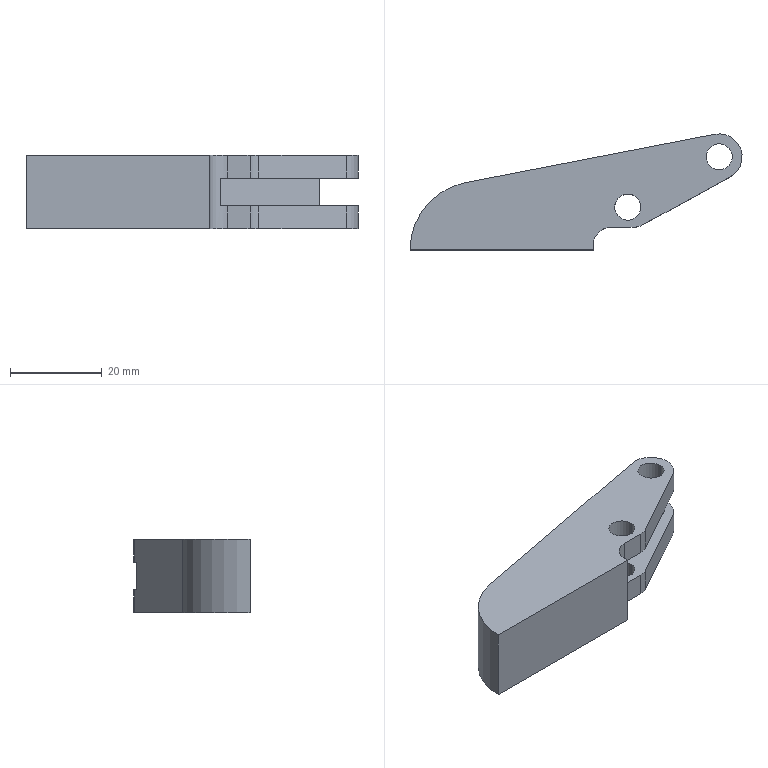Part | SolidWorks | features BaseBody 1, ICE 1, MoveFace 1 | 1 solid | 27 faces | box 72.59 x 25.381 x 16 mm | volume 14653 mm3 | cylinder 14 | plane 13 | commonest cylinder face diameters 5.7 x8 8 x3 10 x2 30 x1
STEP:
#1=CARTESIAN_POINT('',(70.44,20.381,5.));
#2=VERTEX_POINT('',#1);
#3=CARTESIAN_POINT('',(64.74,20.381,5.));
#4=VERTEX_POINT('',#3);
#5=CARTESIAN_POINT('',(67.59,20.381,5.));
#6=DIRECTION('',(0.,0.,-1.));
#7=DIRECTION('',(1.,0.,0.));
#8=AXIS2_PLACEMENT_3D('',#5,#6,#7);
#9=CIRCLE('',#8,2.85);
#10=EDGE_CURVE('',#2,#4,#9,.T.);
#11=ORIENTED_EDGE('',*,*,#10,.F.);
#12=CARTESIAN_POINT('',(70.44,20.381,0.));
#13=VERTEX_POINT('',#12);
#14=CARTESIAN_POINT('',(70.44,20.381,5.));
#15=DIRECTION('',(0.,0.,-1.));
#16=VECTOR('',#15,1000.);
#17=LINE('',#14,#16);
#18=EDGE_CURVE('',#2,#13,#17,.T.);
#19=ORIENTED_EDGE('',*,*,#18,.T.);
#20=CARTESIAN_POINT('',(64.74,20.381,0.));
#21=VERTEX_POINT('',#20);
#22=CARTESIAN_POINT('',(67.59,20.381,0.));
#23=DIRECTION('',(0.,0.,-1.));
#24=DIRECTION('',(1.,0.,0.));
#25=AXIS2_PLACEMENT_3D('',#22,#23,#24);
#26=CIRCLE('',#25,2.85);
#27=EDGE_CURVE('',#13,#21,#26,.T.);
#28=ORIENTED_EDGE('',*,*,#27,.T.);
#29=CARTESIAN_POINT('',(64.74,20.381,5.));
#30=DIRECTION('',(0.,0.,-1.));
#31=VECTOR('',#30,1000.);
#32=LINE('',#29,#31);
#33=EDGE_CURVE('',#4,#21,#32,.T.);
#34=ORIENTED_EDGE('',*,*,#33,.F.);
#35=EDGE_LOOP('',(#11,#19,#28,#34));
#36=FACE_OUTER_BOUND('',#35,.T.);
#37=CARTESIAN_POINT('',(67.59,20.381,5.));
#38=DIRECTION('',(0.,0.,-1.));
#39=DIRECTION('',(-1.,0.,0.));
#40=AXIS2_PLACEMENT_3D('',#37,#38,#39);
#41=CYLINDRICAL_SURFACE('',#40,2.85);
#42=ADVANCED_FACE('',(#36),#41,.F.);
#43=CARTESIAN_POINT('',(50.44,9.381,5.));
#44=VERTEX_POINT('',#43);
#45=CARTESIAN_POINT('',(44.74,9.381,5.));
#46=VERTEX_POINT('',#45);
#47=CARTESIAN_POINT('',(47.59,9.381,5.));
#48=DIRECTION('',(0.,0.,-1.));
#49=DIRECTION('',(1.,0.,0.));
#50=AXIS2_PLACEMENT_3D('',#47,#48,#49);
#51=CIRCLE('',#50,2.85);
#52=EDGE_CURVE('',#44,#46,#51,.T.);
#53=ORIENTED_EDGE('',*,*,#52,.F.);
#54=CARTESIAN_POINT('',(50.44,9.381,0.));
#55=VERTEX_POINT('',#54);
#56=CARTESIAN_POINT('',(50.44,9.381,5.));
#57=DIRECTION('',(0.,0.,-1.));
#58=VECTOR('',#57,1000.);
#59=LINE('',#56,#58);
#60=EDGE_CURVE('',#44,#55,#59,.T.);
#61=ORIENTED_EDGE('',*,*,#60,.T.);
#62=CARTESIAN_POINT('',(44.74,9.381,0.));
#63=VERTEX_POINT('',#62);
#64=CARTESIAN_POINT('',(47.59,9.381,0.));
#65=DIRECTION('',(0.,0.,-1.));
#66=DIRECTION('',(1.,0.,0.));
#67=AXIS2_PLACEMENT_3D('',#64,#65,#66);
#68=CIRCLE('',#67,2.85);
#69=EDGE_CURVE('',#55,#63,#68,.T.);
#70=ORIENTED_EDGE('',*,*,#69,.T.);
#71=CARTESIAN_POINT('',(44.74,9.381,5.));
#72=DIRECTION('',(0.,0.,-1.));
#73=VECTOR('',#72,1000.);
#74=LINE('',#71,#73);
#75=EDGE_CURVE('',#46,#63,#74,.T.);
#76=ORIENTED_EDGE('',*,*,#75,.F.);
#77=EDGE_LOOP('',(#53,#61,#70,#76));
#78=FACE_OUTER_BOUND('',#77,.T.);
#79=CARTESIAN_POINT('',(47.59,9.381,5.));
#80=DIRECTION('',(0.,0.,-1.));
#81=DIRECTION('',(-1.,0.,0.));
#82=AXIS2_PLACEMENT_3D('',#79,#80,#81);
#83=CYLINDRICAL_SURFACE('',#82,2.85);
#84=ADVANCED_FACE('',(#78),#83,.F.);
#85=CARTESIAN_POINT('',(64.74,20.381,16.));
#86=VERTEX_POINT('',#85);
#87=CARTESIAN_POINT('',(70.44,20.381,16.));
#88=VERTEX_POINT('',#87);
#89=CARTESIAN_POINT('',(67.59,20.381,16.));
#90=DIRECTION('',(0.,0.,1.));
#91=DIRECTION('',(1.,0.,0.));
#92=AXIS2_PLACEMENT_3D('',#89,#90,#91);
#93=CIRCLE('',#92,2.85);
#94=EDGE_CURVE('',#86,#88,#93,.T.);
#95=ORIENTED_EDGE('',*,*,#94,.T.);
#96=CARTESIAN_POINT('',(70.44,20.381,11.));
#97=VERTEX_POINT('',#96);
#98=CARTESIAN_POINT('',(70.44,20.381,16.));
#99=DIRECTION('',(0.,0.,-1.));
#100=VECTOR('',#99,1000.);
#101=LINE('',#98,#100);
#102=EDGE_CURVE('',#88,#97,#101,.T.);
#103=ORIENTED_EDGE('',*,*,#102,.T.);
#104=CARTESIAN_POINT('',(64.74,20.381,11.));
#105=VERTEX_POINT('',#104);
#106=CARTESIAN_POINT('',(67.59,20.381,11.));
#107=DIRECTION('',(0.,0.,-1.));
#108=DIRECTION('',(-1.,0.,0.));
#109=AXIS2_PLACEMENT_3D('',#106,#107,#108);
#110=CIRCLE('',#109,2.85);
#111=EDGE_CURVE('',#97,#105,#110,.T.);
#112=ORIENTED_EDGE('',*,*,#111,.T.);
#113=CARTESIAN_POINT('',(64.74,20.381,16.));
#114=DIRECTION('',(0.,0.,-1.));
#115=VECTOR('',#114,1000.);
#116=LINE('',#113,#115);
#117=EDGE_CURVE('',#86,#105,#116,.T.);
#118=ORIENTED_EDGE('',*,*,#117,.F.);
#119=EDGE_LOOP('',(#95,#103,#112,#118));
#120=FACE_OUTER_BOUND('',#119,.T.);
#121=CARTESIAN_POINT('',(67.59,20.381,16.));
#122=DIRECTION('',(0.,0.,-1.));
#123=DIRECTION('',(-1.,0.,0.));
#124=AXIS2_PLACEMENT_3D('',#121,#122,#123);
#125=CYLINDRICAL_SURFACE('',#124,2.85);
#126=ADVANCED_FACE('',(#120),#125,.F.);
#127=CARTESIAN_POINT('',(44.74,9.381,16.));
#128=VERTEX_POINT('',#127);
#129=CARTESIAN_POINT('',(50.44,9.381,16.));
#130=VERTEX_POINT('',#129);
#131=CARTESIAN_POINT('',(47.59,9.381,16.));
#132=DIRECTION('',(0.,0.,1.));
#133=DIRECTION('',(1.,0.,0.));
#134=AXIS2_PLACEMENT_3D('',#131,#132,#133);
#135=CIRCLE('',#134,2.85);
#136=EDGE_CURVE('',#128,#130,#135,.T.);
#137=ORIENTED_EDGE('',*,*,#136,.T.);
#138=CARTESIAN_POINT('',(50.44,9.381,11.));
#139=VERTEX_POINT('',#138);
#140=CARTESIAN_POINT('',(50.44,9.381,16.));
#141=DIRECTION('',(0.,0.,-1.));
#142=VECTOR('',#141,1000.);
#143=LINE('',#140,#142);
#144=EDGE_CURVE('',#130,#139,#143,.T.);
#145=ORIENTED_EDGE('',*,*,#144,.T.);
#146=CARTESIAN_POINT('',(44.74,9.381,11.));
#147=VERTEX_POINT('',#146);
#148=CARTESIAN_POINT('',(47.59,9.381,11.));
#149=DIRECTION('',(0.,0.,-1.));
#150=DIRECTION('',(-1.,0.,0.));
#151=AXIS2_PLACEMENT_3D('',#148,#149,#150);
#152=CIRCLE('',#151,2.85);
#153=EDGE_CURVE('',#139,#147,#152,.T.);
#154=ORIENTED_EDGE('',*,*,#153,.T.);
#155=CARTESIAN_POINT('',(44.74,9.381,16.));
#156=DIRECTION('',(0.,0.,-1.));
#157=VECTOR('',#156,1000.);
#158=LINE('',#155,#157);
#159=EDGE_CURVE('',#128,#147,#158,.T.);
#160=ORIENTED_EDGE('',*,*,#159,.F.);
#161=EDGE_LOOP('',(#137,#145,#154,#160));
#162=FACE_OUTER_BOUND('',#161,.T.);
#163=CARTESIAN_POINT('',(47.59,9.381,16.));
#164=DIRECTION('',(0.,0.,-1.));
#165=DIRECTION('',(-1.,0.,0.));
#166=AXIS2_PLACEMENT_3D('',#163,#164,#165);
#167=CYLINDRICAL_SURFACE('',#166,2.85);
#168=ADVANCED_FACE('',(#162),#167,.F.);
#169=CARTESIAN_POINT('',(42.59,12.922,5.));
#170=VERTEX_POINT('',#169);
#171=CARTESIAN_POINT('',(64.228,24.822,5.));
#172=VERTEX_POINT('',#171);
#173=CARTESIAN_POINT('',(45.834,14.706,5.));
#174=DIRECTION('',(0.8762,0.4819,0.));
#175=VECTOR('',#174,1000.);
#176=LINE('',#173,#175);
#177=EDGE_CURVE('',#170,#172,#176,.T.);
#178=ORIENTED_EDGE('',*,*,#177,.T.);
#179=CARTESIAN_POINT('',(64.228,24.822,11.));
#180=VERTEX_POINT('',#179);
#181=CARTESIAN_POINT('',(64.228,24.822,16.));
#182=DIRECTION('',(0.,0.,1.));
#183=VECTOR('',#182,1000.);
#184=LINE('',#181,#183);
#185=EDGE_CURVE('',#172,#180,#184,.T.);
#186=ORIENTED_EDGE('',*,*,#185,.T.);
#187=CARTESIAN_POINT('',(42.59,12.922,11.));
#188=VERTEX_POINT('',#187);
#189=CARTESIAN_POINT('',(86.688,37.175,11.));
#190=DIRECTION('',(0.8762,0.4819,0.));
#191=VECTOR('',#190,1000.);
#192=LINE('',#189,#191);
#193=EDGE_CURVE('',#188,#180,#192,.T.);
#194=ORIENTED_EDGE('',*,*,#193,.F.);
#195=CARTESIAN_POINT('',(42.59,12.922,11.));
#196=DIRECTION('',(0.,0.,1.));
#197=VECTOR('',#196,1000.);
#198=LINE('',#195,#197);
#199=EDGE_CURVE('',#170,#188,#198,.T.);
#200=ORIENTED_EDGE('',*,*,#199,.F.);
#201=EDGE_LOOP('',(#178,#186,#194,#200));
#202=FACE_OUTER_BOUND('',#201,.T.);
#203=CARTESIAN_POINT('',(45.834,14.706,16.));
#204=DIRECTION('',(-0.4819,0.8762,0.));
#205=DIRECTION('',(-0.8762,-0.4819,0.));
#206=AXIS2_PLACEMENT_3D('',#203,#204,#205);
#207=PLANE('',#206);
#208=ADVANCED_FACE('',(#202),#207,.F.);
#209=CARTESIAN_POINT('',(47.59,9.381,11.));
#210=DIRECTION('',(0.,0.,-1.));
#211=DIRECTION('',(-1.,0.,0.));
#212=AXIS2_PLACEMENT_3D('',#209,#210,#211);
#213=CIRCLE('',#212,2.85);
#214=EDGE_CURVE('',#147,#139,#213,.T.);
#215=ORIENTED_EDGE('',*,*,#214,.F.);
#216=ORIENTED_EDGE('',*,*,#153,.F.);
#217=EDGE_LOOP('',(#215,#216));
#218=FACE_BOUND('',#217,.T.);
#219=CARTESIAN_POINT('',(67.59,20.381,11.));
#220=DIRECTION('',(0.,0.,-1.));
#221=DIRECTION('',(-1.,0.,0.));
#222=AXIS2_PLACEMENT_3D('',#219,#220,#221);
#223=CIRCLE('',#222,2.85);
#224=EDGE_CURVE('',#105,#97,#223,.T.);
#225=ORIENTED_EDGE('',*,*,#224,.F.);
#226=ORIENTED_EDGE('',*,*,#111,.F.);
#227=EDGE_LOOP('',(#225,#226));
#228=FACE_BOUND('',#227,.T.);
#229=CARTESIAN_POINT('',(66.639,25.29,11.));
#230=VERTEX_POINT('',#229);
#231=CARTESIAN_POINT('',(12.145,14.726,11.));
#232=DIRECTION('',(-0.9817,-0.1903,0.));
#233=VECTOR('',#232,1000.);
#234=LINE('',#231,#233);
#235=EDGE_CURVE('',#230,#180,#234,.T.);
#236=ORIENTED_EDGE('',*,*,#235,.F.);
#237=CARTESIAN_POINT('',(70.,16.,11.));
#238=VERTEX_POINT('',#237);
#239=CARTESIAN_POINT('',(67.59,20.381,11.));
#240=DIRECTION('',(0.,0.,1.));
#241=DIRECTION('',(-1.,0.,0.));
#242=AXIS2_PLACEMENT_3D('',#239,#240,#241);
#243=CIRCLE('',#242,5.);
#244=EDGE_CURVE('',#238,#230,#243,.T.);
#245=ORIENTED_EDGE('',*,*,#244,.F.);
#246=CARTESIAN_POINT('',(50.9,5.495,11.));
#247=VERTEX_POINT('',#246);
#248=CARTESIAN_POINT('',(50.9,5.495,11.));
#249=DIRECTION('',(-0.8762,-0.4819,0.));
#250=VECTOR('',#249,1000.);
#251=LINE('',#248,#250);
#252=EDGE_CURVE('',#238,#247,#251,.T.);
#253=ORIENTED_EDGE('',*,*,#252,.T.);
#254=CARTESIAN_POINT('',(48.973,5.,11.));
#255=VERTEX_POINT('',#254);
#256=CARTESIAN_POINT('',(48.973,9.,11.));
#257=DIRECTION('',(0.,0.,1.));
#258=DIRECTION('',(-1.,0.,0.));
#259=AXIS2_PLACEMENT_3D('',#256,#257,#258);
#260=CIRCLE('',#259,4.);
#261=EDGE_CURVE('',#255,#247,#260,.T.);
#262=ORIENTED_EDGE('',*,*,#261,.F.);
#263=CARTESIAN_POINT('',(44.,5.,11.));
#264=VERTEX_POINT('',#263);
#265=CARTESIAN_POINT('',(44.,5.,11.));
#266=DIRECTION('',(-1.,0.,0.));
#267=VECTOR('',#266,1000.);
#268=LINE('',#265,#267);
#269=EDGE_CURVE('',#255,#264,#268,.T.);
#270=ORIENTED_EDGE('',*,*,#269,.T.);
#271=CARTESIAN_POINT('',(42.59,4.743,11.));
#272=VERTEX_POINT('',#271);
#273=CARTESIAN_POINT('',(44.,1.,11.));
#274=DIRECTION('',(0.,0.,1.));
#275=DIRECTION('',(-1.,0.,0.));
#276=AXIS2_PLACEMENT_3D('',#273,#274,#275);
#277=CIRCLE('',#276,4.);
#278=EDGE_CURVE('',#264,#272,#277,.T.);
#279=ORIENTED_EDGE('',*,*,#278,.T.);
#280=CARTESIAN_POINT('',(42.59,62.807,11.));
#281=DIRECTION('',(0.,-1.,0.));
#282=VECTOR('',#281,1000.);
#283=LINE('',#280,#282);
#284=EDGE_CURVE('',#188,#272,#283,.T.);
#285=ORIENTED_EDGE('',*,*,#284,.F.);
#286=ORIENTED_EDGE('',*,*,#193,.T.);
#287=EDGE_LOOP('',(#236,#245,#253,#262,#270,#279,#285,#286));
#288=FACE_OUTER_BOUND('',#287,.T.);
#289=CARTESIAN_POINT('',(72.59,62.807,11.));
#290=DIRECTION('',(0.,0.,-1.));
#291=DIRECTION('',(-1.,0.,0.));
#292=AXIS2_PLACEMENT_3D('',#289,#290,#291);
#293=PLANE('',#292);
#294=ADVANCED_FACE('',(#218,#228,#288),#293,.T.);
#295=CARTESIAN_POINT('',(67.59,20.381,5.));
#296=DIRECTION('',(0.,0.,-1.));
#297=DIRECTION('',(1.,0.,0.));
#298=AXIS2_PLACEMENT_3D('',#295,#296,#297);
#299=CIRCLE('',#298,2.85);
#300=EDGE_CURVE('',#4,#2,#299,.T.);
#301=ORIENTED_EDGE('',*,*,#300,.T.);
#302=ORIENTED_EDGE('',*,*,#10,.T.);
#303=EDGE_LOOP('',(#301,#302));
#304=FACE_BOUND('',#303,.T.);
#305=CARTESIAN_POINT('',(47.59,9.381,5.));
#306=DIRECTION('',(0.,0.,-1.));
#307=DIRECTION('',(1.,0.,0.));
#308=AXIS2_PLACEMENT_3D('',#305,#306,#307);
#309=CIRCLE('',#308,2.85);
#310=EDGE_CURVE('',#46,#44,#309,.T.);
#311=ORIENTED_EDGE('',*,*,#310,.T.);
#312=ORIENTED_EDGE('',*,*,#52,.T.);
#313=EDGE_LOOP('',(#311,#312));
#314=FACE_BOUND('',#313,.T.);
#315=CARTESIAN_POINT('',(66.639,25.29,5.));
#316=VERTEX_POINT('',#315);
#317=CARTESIAN_POINT('',(70.,16.,5.));
#318=VERTEX_POINT('',#317);
#319=CARTESIAN_POINT('',(67.59,20.381,5.));
#320=DIRECTION('',(0.,0.,-1.));
#321=DIRECTION('',(-1.,0.,0.));
#322=AXIS2_PLACEMENT_3D('',#319,#320,#321);
#323=CIRCLE('',#322,5.);
#324=EDGE_CURVE('',#316,#318,#323,.T.);
#325=ORIENTED_EDGE('',*,*,#324,.F.);
#326=CARTESIAN_POINT('',(40.282,20.18,5.));
#327=DIRECTION('',(-0.9817,-0.1903,0.));
#328=VECTOR('',#327,1000.);
#329=LINE('',#326,#328);
#330=EDGE_CURVE('',#316,#172,#329,.T.);
#331=ORIENTED_EDGE('',*,*,#330,.T.);
#332=ORIENTED_EDGE('',*,*,#177,.F.);
#333=CARTESIAN_POINT('',(42.59,4.743,5.));
#334=VERTEX_POINT('',#333);
#335=CARTESIAN_POINT('',(42.59,4.743,5.));
#336=DIRECTION('',(0.,1.,0.));
#337=VECTOR('',#336,1000.);
#338=LINE('',#335,#337);
#339=EDGE_CURVE('',#334,#170,#338,.T.);
#340=ORIENTED_EDGE('',*,*,#339,.F.);
#341=CARTESIAN_POINT('',(44.,5.,5.));
#342=VERTEX_POINT('',#341);
#343=CARTESIAN_POINT('',(44.,1.,5.));
#344=DIRECTION('',(0.,0.,1.));
#345=DIRECTION('',(1.,0.,0.));
#346=AXIS2_PLACEMENT_3D('',#343,#344,#345);
#347=CIRCLE('',#346,4.);
#348=EDGE_CURVE('',#342,#334,#347,.T.);
#349=ORIENTED_EDGE('',*,*,#348,.F.);
#350=CARTESIAN_POINT('',(48.973,5.,5.));
#351=VERTEX_POINT('',#350);
#352=CARTESIAN_POINT('',(48.973,5.,5.));
#353=DIRECTION('',(-1.,0.,0.));
#354=VECTOR('',#353,1000.);
#355=LINE('',#352,#354);
#356=EDGE_CURVE('',#351,#342,#355,.T.);
#357=ORIENTED_EDGE('',*,*,#356,.F.);
#358=CARTESIAN_POINT('',(50.9,5.495,5.));
#359=VERTEX_POINT('',#358);
#360=CARTESIAN_POINT('',(48.973,9.,5.));
#361=DIRECTION('',(0.,0.,-1.));
#362=DIRECTION('',(-1.,0.,0.));
#363=AXIS2_PLACEMENT_3D('',#360,#361,#362);
#364=CIRCLE('',#363,4.);
#365=EDGE_CURVE('',#359,#351,#364,.T.);
#366=ORIENTED_EDGE('',*,*,#365,.F.);
#367=CARTESIAN_POINT('',(70.,16.,5.));
#368=DIRECTION('',(-0.8762,-0.4819,0.));
#369=VECTOR('',#368,1000.);
#370=LINE('',#367,#369);
#371=EDGE_CURVE('',#318,#359,#370,.T.);
#372=ORIENTED_EDGE('',*,*,#371,.F.);
#373=EDGE_LOOP('',(#325,#331,#332,#340,#349,#357,#366,#372));
#374=FACE_OUTER_BOUND('',#373,.T.);
#375=CARTESIAN_POINT('',(44.,1.,5.));
#376=DIRECTION('',(0.,0.,1.));
#377=DIRECTION('',(1.,0.,0.));
#378=AXIS2_PLACEMENT_3D('',#375,#376,#377);
#379=PLANE('',#378);
#380=ADVANCED_FACE('',(#304,#314,#374),#379,.T.);
#381=ORIENTED_EDGE('',*,*,#244,.T.);
#382=CARTESIAN_POINT('',(66.639,25.29,16.));
#383=VERTEX_POINT('',#382);
#384=CARTESIAN_POINT('',(66.639,25.29,16.));
#385=DIRECTION('',(0.,0.,-1.));
#386=VECTOR('',#385,1000.);
#387=LINE('',#384,#386);
#388=EDGE_CURVE('',#383,#230,#387,.T.);
#389=ORIENTED_EDGE('',*,*,#388,.F.);
#390=CARTESIAN_POINT('',(70.,16.,16.));
#391=VERTEX_POINT('',#390);
#392=CARTESIAN_POINT('',(67.59,20.381,16.));
#393=DIRECTION('',(0.,0.,-1.));
#394=DIRECTION('',(-1.,0.,0.));
#395=AXIS2_PLACEMENT_3D('',#392,#393,#394);
#396=CIRCLE('',#395,5.);
#397=EDGE_CURVE('',#383,#391,#396,.T.);
#398=ORIENTED_EDGE('',*,*,#397,.T.);
#399=CARTESIAN_POINT('',(70.,16.,16.));
#400=DIRECTION('',(0.,0.,-1.));
#401=VECTOR('',#400,1000.);
#402=LINE('',#399,#401);
#403=EDGE_CURVE('',#391,#238,#402,.T.);
#404=ORIENTED_EDGE('',*,*,#403,.T.);
#405=EDGE_LOOP('',(#381,#389,#398,#404));
#406=FACE_OUTER_BOUND('',#405,.T.);
#407=CARTESIAN_POINT('',(67.59,20.381,16.));
#408=DIRECTION('',(0.,0.,-1.));
#409=DIRECTION('',(-1.,0.,0.));
#410=AXIS2_PLACEMENT_3D('',#407,#408,#409);
#411=CYLINDRICAL_SURFACE('',#410,5.);
#412=ADVANCED_FACE('',(#406),#411,.T.);
#413=CARTESIAN_POINT('',(40.,1.,0.));
#414=VERTEX_POINT('',#413);
#415=CARTESIAN_POINT('',(44.,5.,0.));
#416=VERTEX_POINT('',#415);
#417=CARTESIAN_POINT('',(44.,1.,0.));
#418=DIRECTION('',(0.,0.,-1.));
#419=DIRECTION('',(-1.,0.,0.));
#420=AXIS2_PLACEMENT_3D('',#417,#418,#419);
#421=CIRCLE('',#420,4.);
#422=EDGE_CURVE('',#414,#416,#421,.T.);
#423=ORIENTED_EDGE('',*,*,#422,.T.);
#424=CARTESIAN_POINT('',(44.,5.,5.));
#425=DIRECTION('',(0.,0.,-1.));
#426=VECTOR('',#425,1000.);
#427=LINE('',#424,#426);
#428=EDGE_CURVE('',#342,#416,#427,.T.);
#429=ORIENTED_EDGE('',*,*,#428,.F.);
#430=ORIENTED_EDGE('',*,*,#348,.T.);
#431=CARTESIAN_POINT('',(42.59,4.743,16.));
#432=DIRECTION('',(0.,0.,-1.));
#433=VECTOR('',#432,1000.);
#434=LINE('',#431,#433);
#435=EDGE_CURVE('',#272,#334,#434,.T.);
#436=ORIENTED_EDGE('',*,*,#435,.F.);
#437=ORIENTED_EDGE('',*,*,#278,.F.);
#438=CARTESIAN_POINT('',(44.,5.,16.));
#439=VERTEX_POINT('',#438);
#440=CARTESIAN_POINT('',(44.,5.,16.));
#441=DIRECTION('',(0.,0.,-1.));
#442=VECTOR('',#441,1000.);
#443=LINE('',#440,#442);
#444=EDGE_CURVE('',#439,#264,#443,.T.);
#445=ORIENTED_EDGE('',*,*,#444,.F.);
#446=CARTESIAN_POINT('',(40.,1.,16.));
#447=VERTEX_POINT('',#446);
#448=CARTESIAN_POINT('',(44.,1.,16.));
#449=DIRECTION('',(0.,0.,-1.));
#450=DIRECTION('',(-1.,0.,0.));
#451=AXIS2_PLACEMENT_3D('',#448,#449,#450);
#452=CIRCLE('',#451,4.);
#453=EDGE_CURVE('',#447,#439,#452,.T.);
#454=ORIENTED_EDGE('',*,*,#453,.F.);
#455=CARTESIAN_POINT('',(40.,1.,16.));
#456=DIRECTION('',(0.,0.,-1.));
#457=VECTOR('',#456,1000.);
#458=LINE('',#455,#457);
#459=EDGE_CURVE('',#447,#414,#458,.T.);
#460=ORIENTED_EDGE('',*,*,#459,.T.);
#461=EDGE_LOOP('',(#423,#429,#430,#436,#437,#445,#454,#460));
#462=FACE_OUTER_BOUND('',#461,.T.);
#463=CARTESIAN_POINT('',(44.,1.,16.));
#464=DIRECTION('',(0.,0.,-1.));
#465=DIRECTION('',(-1.,0.,0.));
#466=AXIS2_PLACEMENT_3D('',#463,#464,#465);
#467=CYLINDRICAL_SURFACE('',#466,4.);
#468=ADVANCED_FACE('',(#462),#467,.F.);
#469=ORIENTED_EDGE('',*,*,#269,.F.);
#470=CARTESIAN_POINT('',(48.973,5.,16.));
#471=VERTEX_POINT('',#470);
#472=CARTESIAN_POINT('',(48.973,5.,16.));
#473=DIRECTION('',(0.,0.,-1.));
#474=VECTOR('',#473,1000.);
#475=LINE('',#472,#474);
#476=EDGE_CURVE('',#471,#255,#475,.T.);
#477=ORIENTED_EDGE('',*,*,#476,.F.);
#478=CARTESIAN_POINT('',(44.,5.,16.));
#479=DIRECTION('',(1.,0.,0.));
#480=VECTOR('',#479,1000.);
#481=LINE('',#478,#480);
#482=EDGE_CURVE('',#439,#471,#481,.T.);
#483=ORIENTED_EDGE('',*,*,#482,.F.);
#484=ORIENTED_EDGE('',*,*,#444,.T.);
#485=EDGE_LOOP('',(#469,#477,#483,#484));
#486=FACE_OUTER_BOUND('',#485,.T.);
#487=CARTESIAN_POINT('',(44.,5.,16.));
#488=DIRECTION('',(0.,1.,0.));
#489=DIRECTION('',(-1.,0.,0.));
#490=AXIS2_PLACEMENT_3D('',#487,#488,#489);
#491=PLANE('',#490);
#492=ADVANCED_FACE('',(#486),#491,.F.);
#493=ORIENTED_EDGE('',*,*,#476,.T.);
#494=ORIENTED_EDGE('',*,*,#261,.T.);
#495=CARTESIAN_POINT('',(50.9,5.495,16.));
#496=VERTEX_POINT('',#495);
#497=CARTESIAN_POINT('',(50.9,5.495,16.));
#498=DIRECTION('',(0.,0.,-1.));
#499=VECTOR('',#498,1000.);
#500=LINE('',#497,#499);
#501=EDGE_CURVE('',#496,#247,#500,.T.);
#502=ORIENTED_EDGE('',*,*,#501,.F.);
#503=CARTESIAN_POINT('',(48.973,9.,16.));
#504=DIRECTION('',(0.,0.,-1.));
#505=DIRECTION('',(-1.,0.,0.));
#506=AXIS2_PLACEMENT_3D('',#503,#504,#505);
#507=CIRCLE('',#506,4.);
#508=EDGE_CURVE('',#496,#471,#507,.T.);
#509=ORIENTED_EDGE('',*,*,#508,.T.);
#510=EDGE_LOOP('',(#493,#494,#502,#509));
#511=FACE_OUTER_BOUND('',#510,.T.);
#512=CARTESIAN_POINT('',(48.973,9.,16.));
#513=DIRECTION('',(0.,0.,-1.));
#514=DIRECTION('',(-1.,0.,0.));
#515=AXIS2_PLACEMENT_3D('',#512,#513,#514);
#516=CYLINDRICAL_SURFACE('',#515,4.);
#517=ADVANCED_FACE('',(#511),#516,.T.);
#518=ORIENTED_EDGE('',*,*,#252,.F.);
#519=ORIENTED_EDGE('',*,*,#403,.F.);
#520=CARTESIAN_POINT('',(50.9,5.495,16.));
#521=DIRECTION('',(0.8762,0.4819,0.));
#522=VECTOR('',#521,1000.);
#523=LINE('',#520,#522);
#524=EDGE_CURVE('',#496,#391,#523,.T.);
#525=ORIENTED_EDGE('',*,*,#524,.F.);
#526=ORIENTED_EDGE('',*,*,#501,.T.);
#527=EDGE_LOOP('',(#518,#519,#525,#526));
#528=FACE_OUTER_BOUND('',#527,.T.);
#529=CARTESIAN_POINT('',(50.9,5.495,16.));
#530=DIRECTION('',(-0.4819,0.8762,0.));
#531=DIRECTION('',(-0.8762,-0.4819,0.));
#532=AXIS2_PLACEMENT_3D('',#529,#530,#531);
#533=PLANE('',#532);
#534=ADVANCED_FACE('',(#528),#533,.F.);
#535=CARTESIAN_POINT('',(66.639,25.29,0.));
#536=VERTEX_POINT('',#535);
#537=CARTESIAN_POINT('',(66.639,25.29,16.));
#538=DIRECTION('',(0.,0.,-1.));
#539=VECTOR('',#538,1000.);
#540=LINE('',#537,#539);
#541=EDGE_CURVE('',#316,#536,#540,.T.);
#542=ORIENTED_EDGE('',*,*,#541,.F.);
#543=ORIENTED_EDGE('',*,*,#324,.T.);
#544=CARTESIAN_POINT('',(70.,16.,0.));
#545=VERTEX_POINT('',#544);
#546=CARTESIAN_POINT('',(70.,16.,5.));
#547=DIRECTION('',(0.,0.,-1.));
#548=VECTOR('',#547,1000.);
#549=LINE('',#546,#548);
#550=EDGE_CURVE('',#318,#545,#549,.T.);
#551=ORIENTED_EDGE('',*,*,#550,.T.);
#552=CARTESIAN_POINT('',(67.59,20.381,0.));
#553=DIRECTION('',(0.,0.,-1.));
#554=DIRECTION('',(-1.,0.,0.));
#555=AXIS2_PLACEMENT_3D('',#552,#553,#554);
#556=CIRCLE('',#555,5.);
#557=EDGE_CURVE('',#536,#545,#556,.T.);
#558=ORIENTED_EDGE('',*,*,#557,.F.);
#559=EDGE_LOOP('',(#542,#543,#551,#558));
#560=FACE_OUTER_BOUND('',#559,.T.);
#561=CARTESIAN_POINT('',(67.59,20.381,16.));
#562=DIRECTION('',(0.,0.,-1.));
#563=DIRECTION('',(-1.,0.,0.));
#564=AXIS2_PLACEMENT_3D('',#561,#562,#563);
#565=CYLINDRICAL_SURFACE('',#564,5.);
#566=ADVANCED_FACE('',(#560),#565,.T.);
#567=ORIENTED_EDGE('',*,*,#144,.F.);
#568=CARTESIAN_POINT('',(47.59,9.381,16.));
#569=DIRECTION('',(0.,0.,1.));
#570=DIRECTION('',(1.,0.,0.));
#571=AXIS2_PLACEMENT_3D('',#568,#569,#570);
#572=CIRCLE('',#571,2.85);
#573=EDGE_CURVE('',#130,#128,#572,.T.);
#574=ORIENTED_EDGE('',*,*,#573,.T.);
#575=ORIENTED_EDGE('',*,*,#159,.T.);
#576=ORIENTED_EDGE('',*,*,#214,.T.);
#577=EDGE_LOOP('',(#567,#574,#575,#576));
#578=FACE_OUTER_BOUND('',#577,.T.);
#579=CARTESIAN_POINT('',(47.59,9.381,16.));
#580=DIRECTION('',(0.,0.,-1.));
#581=DIRECTION('',(-1.,0.,0.));
#582=AXIS2_PLACEMENT_3D('',#579,#580,#581);
#583=CYLINDRICAL_SURFACE('',#582,2.85);
#584=ADVANCED_FACE('',(#578),#583,.F.);
#585=ORIENTED_EDGE('',*,*,#102,.F.);
#586=CARTESIAN_POINT('',(67.59,20.381,16.));
#587=DIRECTION('',(0.,0.,1.));
#588=DIRECTION('',(1.,0.,0.));
#589=AXIS2_PLACEMENT_3D('',#586,#587,#588);
#590=CIRCLE('',#589,2.85);
#591=EDGE_CURVE('',#88,#86,#590,.T.);
#592=ORIENTED_EDGE('',*,*,#591,.T.);
#593=ORIENTED_EDGE('',*,*,#117,.T.);
#594=ORIENTED_EDGE('',*,*,#224,.T.);
#595=EDGE_LOOP('',(#585,#592,#593,#594));
#596=FACE_OUTER_BOUND('',#595,.T.);
#597=CARTESIAN_POINT('',(67.59,20.381,16.));
#598=DIRECTION('',(0.,0.,-1.));
#599=DIRECTION('',(-1.,0.,0.));
#600=AXIS2_PLACEMENT_3D('',#597,#598,#599);
#601=CYLINDRICAL_SURFACE('',#600,2.85);
#602=ADVANCED_FACE('',(#596),#601,.F.);
#603=ORIENTED_EDGE('',*,*,#136,.F.);
#604=ORIENTED_EDGE('',*,*,#573,.F.);
#605=EDGE_LOOP('',(#603,#604));
#606=FACE_BOUND('',#605,.T.);
#607=CARTESIAN_POINT('',(12.145,14.726,16.));
#608=VERTEX_POINT('',#607);
#609=CARTESIAN_POINT('',(0.,0.,16.));
#610=VERTEX_POINT('',#609);
#611=CARTESIAN_POINT('',(15.,0.,16.));
#612=DIRECTION('',(0.,0.,1.));
#613=DIRECTION('',(1.,0.,0.));
#614=AXIS2_PLACEMENT_3D('',#611,#612,#613);
#615=CIRCLE('',#614,15.);
#616=EDGE_CURVE('',#608,#610,#615,.T.);
#617=ORIENTED_EDGE('',*,*,#616,.T.);
#618=CARTESIAN_POINT('',(40.,0.,16.));
#619=VERTEX_POINT('',#618);
#620=CARTESIAN_POINT('',(0.,0.,16.));
#621=DIRECTION('',(1.,0.,0.));
#622=VECTOR('',#621,1000.);
#623=LINE('',#620,#622);
#624=EDGE_CURVE('',#610,#619,#623,.T.);
#625=ORIENTED_EDGE('',*,*,#624,.T.);
#626=CARTESIAN_POINT('',(40.,0.,16.));
#627=DIRECTION('',(0.,1.,0.));
#628=VECTOR('',#627,1000.);
#629=LINE('',#626,#628);
#630=EDGE_CURVE('',#619,#447,#629,.T.);
#631=ORIENTED_EDGE('',*,*,#630,.T.);
#632=ORIENTED_EDGE('',*,*,#453,.T.);
#633=ORIENTED_EDGE('',*,*,#482,.T.);
#634=ORIENTED_EDGE('',*,*,#508,.F.);
#635=ORIENTED_EDGE('',*,*,#524,.T.);
#636=ORIENTED_EDGE('',*,*,#397,.F.);
#637=CARTESIAN_POINT('',(12.145,14.726,16.));
#638=DIRECTION('',(0.9817,0.1903,0.));
#639=VECTOR('',#638,1000.);
#640=LINE('',#637,#639);
#641=EDGE_CURVE('',#608,#383,#640,.T.);
#642=ORIENTED_EDGE('',*,*,#641,.F.);
#643=EDGE_LOOP('',(#617,#625,#631,#632,#633,#634,#635,#636,#642));
#644=FACE_OUTER_BOUND('',#643,.T.);
#645=ORIENTED_EDGE('',*,*,#94,.F.);
#646=ORIENTED_EDGE('',*,*,#591,.F.);
#647=EDGE_LOOP('',(#645,#646));
#648=FACE_BOUND('',#647,.T.);
#649=CARTESIAN_POINT('',(15.,0.,16.));
#650=DIRECTION('',(0.,0.,1.));
#651=DIRECTION('',(1.,0.,0.));
#652=AXIS2_PLACEMENT_3D('',#649,#650,#651);
#653=PLANE('',#652);
#654=ADVANCED_FACE('',(#606,#644,#648),#653,.T.);
#655=CARTESIAN_POINT('',(48.973,5.,0.));
#656=VERTEX_POINT('',#655);
#657=CARTESIAN_POINT('',(48.973,5.,0.));
#658=DIRECTION('',(-1.,0.,0.));
#659=VECTOR('',#658,1000.);
#660=LINE('',#657,#659);
#661=EDGE_CURVE('',#656,#416,#660,.T.);
#662=ORIENTED_EDGE('',*,*,#661,.T.);
#663=ORIENTED_EDGE('',*,*,#422,.F.);
#664=CARTESIAN_POINT('',(40.,0.,0.));
#665=VERTEX_POINT('',#664);
#666=CARTESIAN_POINT('',(40.,0.,0.));
#667=DIRECTION('',(0.,1.,0.));
#668=VECTOR('',#667,1000.);
#669=LINE('',#666,#668);
#670=EDGE_CURVE('',#665,#414,#669,.T.);
#671=ORIENTED_EDGE('',*,*,#670,.F.);
#672=CARTESIAN_POINT('',(0.,0.,0.));
#673=VERTEX_POINT('',#672);
#674=CARTESIAN_POINT('',(0.,0.,0.));
#675=DIRECTION('',(1.,0.,0.));
#676=VECTOR('',#675,1000.);
#677=LINE('',#674,#676);
#678=EDGE_CURVE('',#673,#665,#677,.T.);
#679=ORIENTED_EDGE('',*,*,#678,.F.);
#680=CARTESIAN_POINT('',(12.145,14.726,0.));
#681=VERTEX_POINT('',#680);
#682=CARTESIAN_POINT('',(15.,0.,0.));
#683=DIRECTION('',(0.,0.,1.));
#684=DIRECTION('',(1.,0.,0.));
#685=AXIS2_PLACEMENT_3D('',#682,#683,#684);
#686=CIRCLE('',#685,15.);
#687=EDGE_CURVE('',#681,#673,#686,.T.);
#688=ORIENTED_EDGE('',*,*,#687,.F.);
#689=CARTESIAN_POINT('',(12.145,14.726,0.));
#690=DIRECTION('',(0.9817,0.1903,0.));
#691=VECTOR('',#690,1000.);
#692=LINE('',#689,#691);
#693=EDGE_CURVE('',#681,#536,#692,.T.);
#694=ORIENTED_EDGE('',*,*,#693,.T.);
#695=ORIENTED_EDGE('',*,*,#557,.T.);
#696=CARTESIAN_POINT('',(50.9,5.495,0.));
#697=VERTEX_POINT('',#696);
#698=CARTESIAN_POINT('',(70.,16.,0.));
#699=DIRECTION('',(-0.8762,-0.4819,0.));
#700=VECTOR('',#699,1000.);
#701=LINE('',#698,#700);
#702=EDGE_CURVE('',#545,#697,#701,.T.);
#703=ORIENTED_EDGE('',*,*,#702,.T.);
#704=CARTESIAN_POINT('',(48.973,9.,0.));
#705=DIRECTION('',(0.,0.,-1.));
#706=DIRECTION('',(-1.,0.,0.));
#707=AXIS2_PLACEMENT_3D('',#704,#705,#706);
#708=CIRCLE('',#707,4.);
#709=EDGE_CURVE('',#697,#656,#708,.T.);
#710=ORIENTED_EDGE('',*,*,#709,.T.);
#711=EDGE_LOOP('',(#662,#663,#671,#679,#688,#694,#695,#703,#710));
#712=FACE_OUTER_BOUND('',#711,.T.);
#713=CARTESIAN_POINT('',(67.59,20.381,0.));
#714=DIRECTION('',(0.,0.,-1.));
#715=DIRECTION('',(1.,0.,0.));
#716=AXIS2_PLACEMENT_3D('',#713,#714,#715);
#717=CIRCLE('',#716,2.85);
#718=EDGE_CURVE('',#21,#13,#717,.T.);
#719=ORIENTED_EDGE('',*,*,#718,.F.);
#720=ORIENTED_EDGE('',*,*,#27,.F.);
#721=EDGE_LOOP('',(#719,#720));
#722=FACE_BOUND('',#721,.T.);
#723=CARTESIAN_POINT('',(47.59,9.381,0.));
#724=DIRECTION('',(0.,0.,-1.));
#725=DIRECTION('',(1.,0.,0.));
#726=AXIS2_PLACEMENT_3D('',#723,#724,#725);
#727=CIRCLE('',#726,2.85);
#728=EDGE_CURVE('',#63,#55,#727,.T.);
#729=ORIENTED_EDGE('',*,*,#728,.F.);
#730=ORIENTED_EDGE('',*,*,#69,.F.);
#731=EDGE_LOOP('',(#729,#730));
#732=FACE_BOUND('',#731,.T.);
#733=CARTESIAN_POINT('',(15.,0.,0.));
#734=DIRECTION('',(0.,0.,1.));
#735=DIRECTION('',(1.,0.,0.));
#736=AXIS2_PLACEMENT_3D('',#733,#734,#735);
#737=PLANE('',#736);
#738=ADVANCED_FACE('',(#712,#722,#732),#737,.F.);
#739=ORIENTED_EDGE('',*,*,#687,.T.);
#740=CARTESIAN_POINT('',(0.,0.,16.));
#741=DIRECTION('',(0.,0.,-1.));
#742=VECTOR('',#741,1000.);
#743=LINE('',#740,#742);
#744=EDGE_CURVE('',#610,#673,#743,.T.);
#745=ORIENTED_EDGE('',*,*,#744,.F.);
#746=ORIENTED_EDGE('',*,*,#616,.F.);
#747=CARTESIAN_POINT('',(12.145,14.726,16.));
#748=DIRECTION('',(0.,0.,-1.));
#749=VECTOR('',#748,1000.);
#750=LINE('',#747,#749);
#751=EDGE_CURVE('',#608,#681,#750,.T.);
#752=ORIENTED_EDGE('',*,*,#751,.T.);
#753=EDGE_LOOP('',(#739,#745,#746,#752));
#754=FACE_OUTER_BOUND('',#753,.T.);
#755=CARTESIAN_POINT('',(15.,0.,16.));
#756=DIRECTION('',(0.,0.,-1.));
#757=DIRECTION('',(-1.,0.,0.));
#758=AXIS2_PLACEMENT_3D('',#755,#756,#757);
#759=CYLINDRICAL_SURFACE('',#758,15.);
#760=ADVANCED_FACE('',(#754),#759,.T.);
#761=ORIENTED_EDGE('',*,*,#678,.T.);
#762=CARTESIAN_POINT('',(40.,0.,16.));
#763=DIRECTION('',(0.,0.,-1.));
#764=VECTOR('',#763,1000.);
#765=LINE('',#762,#764);
#766=EDGE_CURVE('',#619,#665,#765,.T.);
#767=ORIENTED_EDGE('',*,*,#766,.F.);
#768=ORIENTED_EDGE('',*,*,#624,.F.);
#769=ORIENTED_EDGE('',*,*,#744,.T.);
#770=EDGE_LOOP('',(#761,#767,#768,#769));
#771=FACE_OUTER_BOUND('',#770,.T.);
#772=CARTESIAN_POINT('',(0.,0.,16.));
#773=DIRECTION('',(0.,1.,0.));
#774=DIRECTION('',(0.,0.,1.));
#775=AXIS2_PLACEMENT_3D('',#772,#773,#774);
#776=PLANE('',#775);
#777=ADVANCED_FACE('',(#771),#776,.F.);
#778=ORIENTED_EDGE('',*,*,#670,.T.);
#779=ORIENTED_EDGE('',*,*,#459,.F.);
#780=ORIENTED_EDGE('',*,*,#630,.F.);
#781=ORIENTED_EDGE('',*,*,#766,.T.);
#782=EDGE_LOOP('',(#778,#779,#780,#781));
#783=FACE_OUTER_BOUND('',#782,.T.);
#784=CARTESIAN_POINT('',(40.,0.,16.));
#785=DIRECTION('',(-1.,0.,0.));
#786=DIRECTION('',(0.,0.,1.));
#787=AXIS2_PLACEMENT_3D('',#784,#785,#786);
#788=PLANE('',#787);
#789=ADVANCED_FACE('',(#783),#788,.F.);
#790=ORIENTED_EDGE('',*,*,#185,.F.);
#791=ORIENTED_EDGE('',*,*,#330,.F.);
#792=ORIENTED_EDGE('',*,*,#541,.T.);
#793=ORIENTED_EDGE('',*,*,#693,.F.);
#794=ORIENTED_EDGE('',*,*,#751,.F.);
#795=ORIENTED_EDGE('',*,*,#641,.T.);
#796=ORIENTED_EDGE('',*,*,#388,.T.);
#797=ORIENTED_EDGE('',*,*,#235,.T.);
#798=EDGE_LOOP('',(#790,#791,#792,#793,#794,#795,#796,#797));
#799=FACE_OUTER_BOUND('',#798,.T.);
#800=CARTESIAN_POINT('',(12.145,14.726,16.));
#801=DIRECTION('',(-0.1903,0.9817,0.));
#802=DIRECTION('',(-0.9817,-0.1903,0.));
#803=AXIS2_PLACEMENT_3D('',#800,#801,#802);
#804=PLANE('',#803);
#805=ADVANCED_FACE('',(#799),#804,.T.);
#806=ORIENTED_EDGE('',*,*,#339,.T.);
#807=ORIENTED_EDGE('',*,*,#199,.T.);
#808=ORIENTED_EDGE('',*,*,#284,.T.);
#809=ORIENTED_EDGE('',*,*,#435,.T.);
#810=EDGE_LOOP('',(#806,#807,#808,#809));
#811=FACE_OUTER_BOUND('',#810,.T.);
#812=CARTESIAN_POINT('',(42.59,62.807,11.));
#813=DIRECTION('',(1.,0.,0.));
#814=DIRECTION('',(0.,0.,-1.));
#815=AXIS2_PLACEMENT_3D('',#812,#813,#814);
#816=PLANE('',#815);
#817=ADVANCED_FACE('',(#811),#816,.T.);
#818=ORIENTED_EDGE('',*,*,#661,.F.);
#819=CARTESIAN_POINT('',(48.973,5.,5.));
#820=DIRECTION('',(0.,0.,-1.));
#821=VECTOR('',#820,1000.);
#822=LINE('',#819,#821);
#823=EDGE_CURVE('',#351,#656,#822,.T.);
#824=ORIENTED_EDGE('',*,*,#823,.F.);
#825=ORIENTED_EDGE('',*,*,#356,.T.);
#826=ORIENTED_EDGE('',*,*,#428,.T.);
#827=EDGE_LOOP('',(#818,#824,#825,#826));
#828=FACE_OUTER_BOUND('',#827,.T.);
#829=CARTESIAN_POINT('',(48.973,5.,5.));
#830=DIRECTION('',(0.,-1.,0.));
#831=DIRECTION('',(0.,0.,-1.));
#832=AXIS2_PLACEMENT_3D('',#829,#830,#831);
#833=PLANE('',#832);
#834=ADVANCED_FACE('',(#828),#833,.T.);
#835=ORIENTED_EDGE('',*,*,#709,.F.);
#836=CARTESIAN_POINT('',(50.9,5.495,5.));
#837=DIRECTION('',(0.,0.,-1.));
#838=VECTOR('',#837,1000.);
#839=LINE('',#836,#838);
#840=EDGE_CURVE('',#359,#697,#839,.T.);
#841=ORIENTED_EDGE('',*,*,#840,.F.);
#842=ORIENTED_EDGE('',*,*,#365,.T.);
#843=ORIENTED_EDGE('',*,*,#823,.T.);
#844=EDGE_LOOP('',(#835,#841,#842,#843));
#845=FACE_OUTER_BOUND('',#844,.T.);
#846=CARTESIAN_POINT('',(48.973,9.,5.));
#847=DIRECTION('',(0.,0.,-1.));
#848=DIRECTION('',(-1.,0.,0.));
#849=AXIS2_PLACEMENT_3D('',#846,#847,#848);
#850=CYLINDRICAL_SURFACE('',#849,4.);
#851=ADVANCED_FACE('',(#845),#850,.T.);
#852=ORIENTED_EDGE('',*,*,#702,.F.);
#853=ORIENTED_EDGE('',*,*,#550,.F.);
#854=ORIENTED_EDGE('',*,*,#371,.T.);
#855=ORIENTED_EDGE('',*,*,#840,.T.);
#856=EDGE_LOOP('',(#852,#853,#854,#855));
#857=FACE_OUTER_BOUND('',#856,.T.);
#858=CARTESIAN_POINT('',(70.,16.,5.));
#859=DIRECTION('',(0.4819,-0.8762,0.));
#860=DIRECTION('',(0.8762,0.4819,0.));
#861=AXIS2_PLACEMENT_3D('',#858,#859,#860);
#862=PLANE('',#861);
#863=ADVANCED_FACE('',(#857),#862,.T.);
#864=ORIENTED_EDGE('',*,*,#60,.F.);
#865=ORIENTED_EDGE('',*,*,#310,.F.);
#866=ORIENTED_EDGE('',*,*,#75,.T.);
#867=ORIENTED_EDGE('',*,*,#728,.T.);
#868=EDGE_LOOP('',(#864,#865,#866,#867));
#869=FACE_OUTER_BOUND('',#868,.T.);
#870=CARTESIAN_POINT('',(47.59,9.381,5.));
#871=DIRECTION('',(0.,0.,-1.));
#872=DIRECTION('',(-1.,0.,0.));
#873=AXIS2_PLACEMENT_3D('',#870,#871,#872);
#874=CYLINDRICAL_SURFACE('',#873,2.85);
#875=ADVANCED_FACE('',(#869),#874,.F.);
#876=ORIENTED_EDGE('',*,*,#18,.F.);
#877=ORIENTED_EDGE('',*,*,#300,.F.);
#878=ORIENTED_EDGE('',*,*,#33,.T.);
#879=ORIENTED_EDGE('',*,*,#718,.T.);
#880=EDGE_LOOP('',(#876,#877,#878,#879));
#881=FACE_OUTER_BOUND('',#880,.T.);
#882=CARTESIAN_POINT('',(67.59,20.381,5.));
#883=DIRECTION('',(0.,0.,-1.));
#884=DIRECTION('',(-1.,0.,0.));
#885=AXIS2_PLACEMENT_3D('',#882,#883,#884);
#886=CYLINDRICAL_SURFACE('',#885,2.85);
#887=ADVANCED_FACE('',(#881),#886,.F.);
#888=CLOSED_SHELL('',(#42,#84,#126,#168,#208,#294,#380,#412,#468,#492,#517,#534,#566,#584,#602,#654,#738,#760,#777,#789,#805,#817,#834,#851,#863,#875,#887));
#889=MANIFOLD_SOLID_BREP('',#888);
#890=CARTESIAN_POINT('',(0.,0.,0.));
#891=DIRECTION('',(0.,0.,1.));
#892=DIRECTION('',(1.,0.,0.));
#893=AXIS2_PLACEMENT_3D('',#890,#891,#892);
#894=(LENGTH_UNIT()NAMED_UNIT(*)SI_UNIT(.MILLI.,.METRE.));
#895=UNCERTAINTY_MEASURE_WITH_UNIT(LENGTH_MEASURE(0.00001),#894,'','');
#896=(NAMED_UNIT(*)PLANE_ANGLE_UNIT()SI_UNIT($,.RADIAN.));
#897=(NAMED_UNIT(*)SI_UNIT($,.STERADIAN.)SOLID_ANGLE_UNIT());
#898=(GEOMETRIC_REPRESENTATION_CONTEXT(3)GLOBAL_UNCERTAINTY_ASSIGNED_CONTEXT((#895))GLOBAL_UNIT_ASSIGNED_CONTEXT((#894,#896,#897))REPRESENTATION_CONTEXT('',''));
#899=ADVANCED_BREP_SHAPE_REPRESENTATION('',(#889,#893),#898);